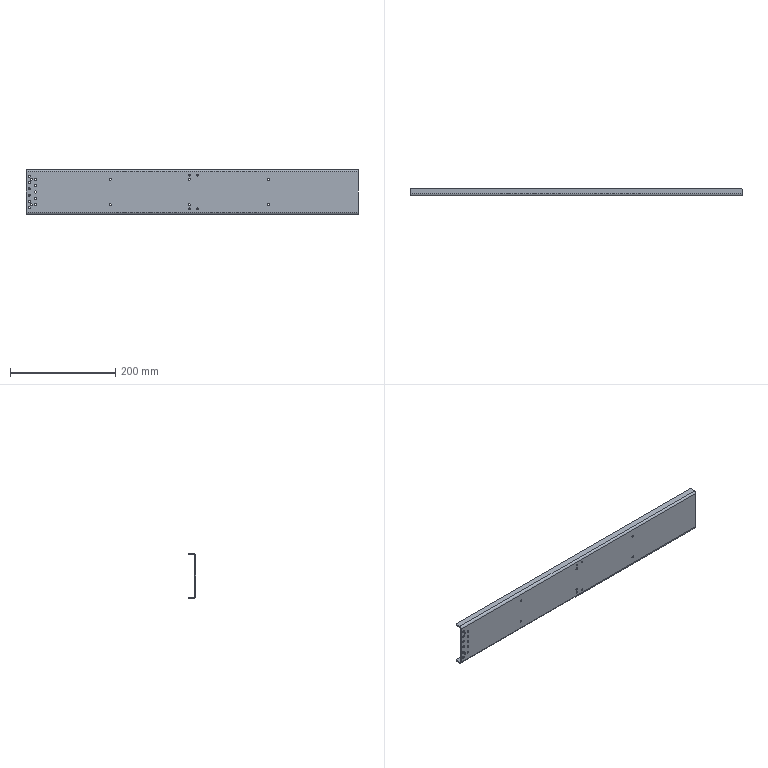Part | SolidWorks | features HoleWzd 3, EdgeFlange 1, Fillet 1, FlatPattern 1, SMBaseFlange 1, SheetMetal 1 | 1 solid | 88 faces | box 630 x 15 x 85 mm | volume 135946 mm3 | cylinder 54 | plane 18 | cone 16 | commonest cylinder face diameters 4.2 x22 3.4 x16 3.3 x8 4 x6 8 x2